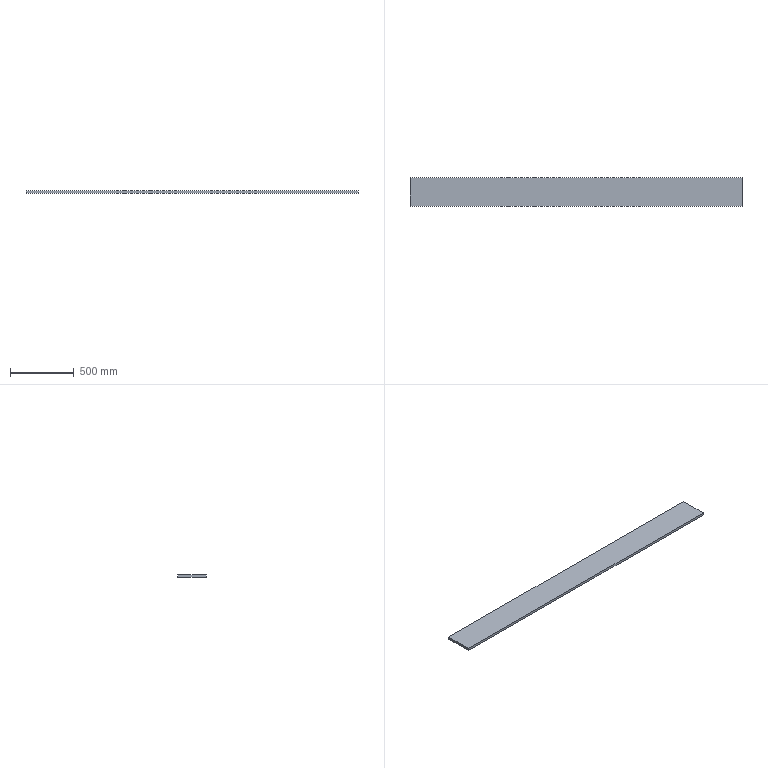Part | NX | features BREP 1, DATUM_CSYS 1, SKETCH 1 | 1 solid | 6 faces | box 2607 x 220 x 20 mm | volume 11470800 mm3 | plane 6
STEP:
#1=CARTESIAN_POINT('',(-1303.5,110.,-10.));
#2=VERTEX_POINT('',#1);
#3=CARTESIAN_POINT('',(-1303.5,-110.,-10.));
#4=VERTEX_POINT('',#3);
#5=CARTESIAN_POINT('',(-1303.5,110.,-10.));
#6=DIRECTION('',(0.,-1.,0.));
#7=VECTOR('',#6,1000.);
#8=LINE('',#5,#7);
#9=EDGE_CURVE('',#2,#4,#8,.T.);
#10=ORIENTED_EDGE('',*,*,#9,.T.);
#11=CARTESIAN_POINT('',(-1303.5,-110.,10.));
#12=VERTEX_POINT('',#11);
#13=CARTESIAN_POINT('',(-1303.5,-110.,10.));
#14=DIRECTION('',(0.,0.,-1.));
#15=VECTOR('',#14,1000.);
#16=LINE('',#13,#15);
#17=EDGE_CURVE('',#12,#4,#16,.T.);
#18=ORIENTED_EDGE('',*,*,#17,.F.);
#19=CARTESIAN_POINT('',(-1303.5,110.,10.));
#20=VERTEX_POINT('',#19);
#21=CARTESIAN_POINT('',(-1303.5,110.,10.));
#22=DIRECTION('',(0.,-1.,0.));
#23=VECTOR('',#22,1000.);
#24=LINE('',#21,#23);
#25=EDGE_CURVE('',#20,#12,#24,.T.);
#26=ORIENTED_EDGE('',*,*,#25,.F.);
#27=CARTESIAN_POINT('',(-1303.5,110.,10.));
#28=DIRECTION('',(0.,0.,-1.));
#29=VECTOR('',#28,1000.);
#30=LINE('',#27,#29);
#31=EDGE_CURVE('',#20,#2,#30,.T.);
#32=ORIENTED_EDGE('',*,*,#31,.T.);
#33=EDGE_LOOP('',(#10,#18,#26,#32));
#34=FACE_BOUND('',#33,.T.);
#35=CARTESIAN_POINT('',(-1303.5,110.,10.));
#36=DIRECTION('',(1.,0.,0.));
#37=DIRECTION('',(0.,0.,1.));
#38=AXIS2_PLACEMENT_3D('',#35,#36,#37);
#39=PLANE('',#38);
#40=ADVANCED_FACE('',(#34),#39,.F.);
#41=CARTESIAN_POINT('',(1303.5,-110.,-10.));
#42=VERTEX_POINT('',#41);
#43=CARTESIAN_POINT('',(-1303.5,-110.,-10.));
#44=DIRECTION('',(1.,0.,0.));
#45=VECTOR('',#44,1000.);
#46=LINE('',#43,#45);
#47=EDGE_CURVE('',#4,#42,#46,.T.);
#48=ORIENTED_EDGE('',*,*,#47,.T.);
#49=CARTESIAN_POINT('',(1303.5,-110.,10.));
#50=VERTEX_POINT('',#49);
#51=CARTESIAN_POINT('',(1303.5,-110.,10.));
#52=DIRECTION('',(0.,0.,-1.));
#53=VECTOR('',#52,1000.);
#54=LINE('',#51,#53);
#55=EDGE_CURVE('',#50,#42,#54,.T.);
#56=ORIENTED_EDGE('',*,*,#55,.F.);
#57=CARTESIAN_POINT('',(-1303.5,-110.,10.));
#58=DIRECTION('',(1.,0.,0.));
#59=VECTOR('',#58,1000.);
#60=LINE('',#57,#59);
#61=EDGE_CURVE('',#12,#50,#60,.T.);
#62=ORIENTED_EDGE('',*,*,#61,.F.);
#63=ORIENTED_EDGE('',*,*,#17,.T.);
#64=EDGE_LOOP('',(#48,#56,#62,#63));
#65=FACE_BOUND('',#64,.T.);
#66=CARTESIAN_POINT('',(-1303.5,-110.,10.));
#67=DIRECTION('',(0.,1.,0.));
#68=DIRECTION('',(0.,0.,-1.));
#69=AXIS2_PLACEMENT_3D('',#66,#67,#68);
#70=PLANE('',#69);
#71=ADVANCED_FACE('',(#65),#70,.F.);
#72=CARTESIAN_POINT('',(1303.5,110.,-10.));
#73=VERTEX_POINT('',#72);
#74=CARTESIAN_POINT('',(1303.5,110.,-10.));
#75=DIRECTION('',(0.,1.,0.));
#76=VECTOR('',#75,1000.);
#77=LINE('',#74,#76);
#78=EDGE_CURVE('',#42,#73,#77,.T.);
#79=ORIENTED_EDGE('',*,*,#78,.T.);
#80=CARTESIAN_POINT('',(1303.5,110.,10.));
#81=VERTEX_POINT('',#80);
#82=CARTESIAN_POINT('',(1303.5,110.,10.));
#83=DIRECTION('',(0.,0.,-1.));
#84=VECTOR('',#83,1000.);
#85=LINE('',#82,#84);
#86=EDGE_CURVE('',#81,#73,#85,.T.);
#87=ORIENTED_EDGE('',*,*,#86,.F.);
#88=CARTESIAN_POINT('',(1303.5,110.,10.));
#89=DIRECTION('',(0.,1.,0.));
#90=VECTOR('',#89,1000.);
#91=LINE('',#88,#90);
#92=EDGE_CURVE('',#50,#81,#91,.T.);
#93=ORIENTED_EDGE('',*,*,#92,.F.);
#94=ORIENTED_EDGE('',*,*,#55,.T.);
#95=EDGE_LOOP('',(#79,#87,#93,#94));
#96=FACE_BOUND('',#95,.T.);
#97=CARTESIAN_POINT('',(1303.5,110.,10.));
#98=DIRECTION('',(-1.,0.,0.));
#99=DIRECTION('',(0.,0.,-1.));
#100=AXIS2_PLACEMENT_3D('',#97,#98,#99);
#101=PLANE('',#100);
#102=ADVANCED_FACE('',(#96),#101,.F.);
#103=CARTESIAN_POINT('',(-1303.5,110.,-10.));
#104=DIRECTION('',(-1.,0.,0.));
#105=VECTOR('',#104,1000.);
#106=LINE('',#103,#105);
#107=EDGE_CURVE('',#73,#2,#106,.T.);
#108=ORIENTED_EDGE('',*,*,#107,.T.);
#109=ORIENTED_EDGE('',*,*,#31,.F.);
#110=CARTESIAN_POINT('',(-1303.5,110.,10.));
#111=DIRECTION('',(-1.,0.,0.));
#112=VECTOR('',#111,1000.);
#113=LINE('',#110,#112);
#114=EDGE_CURVE('',#81,#20,#113,.T.);
#115=ORIENTED_EDGE('',*,*,#114,.F.);
#116=ORIENTED_EDGE('',*,*,#86,.T.);
#117=EDGE_LOOP('',(#108,#109,#115,#116));
#118=FACE_BOUND('',#117,.T.);
#119=CARTESIAN_POINT('',(-1303.5,110.,10.));
#120=DIRECTION('',(0.,-1.,0.));
#121=DIRECTION('',(0.,0.,1.));
#122=AXIS2_PLACEMENT_3D('',#119,#120,#121);
#123=PLANE('',#122);
#124=ADVANCED_FACE('',(#118),#123,.F.);
#125=ORIENTED_EDGE('',*,*,#25,.T.);
#126=ORIENTED_EDGE('',*,*,#61,.T.);
#127=ORIENTED_EDGE('',*,*,#92,.T.);
#128=ORIENTED_EDGE('',*,*,#114,.T.);
#129=EDGE_LOOP('',(#125,#126,#127,#128));
#130=FACE_BOUND('',#129,.T.);
#131=CARTESIAN_POINT('',(-1303.5,-110.,10.));
#132=DIRECTION('',(0.,0.,1.));
#133=DIRECTION('',(-1.,0.,0.));
#134=AXIS2_PLACEMENT_3D('',#131,#132,#133);
#135=PLANE('',#134);
#136=ADVANCED_FACE('',(#130),#135,.T.);
#137=ORIENTED_EDGE('',*,*,#9,.F.);
#138=ORIENTED_EDGE('',*,*,#107,.F.);
#139=ORIENTED_EDGE('',*,*,#78,.F.);
#140=ORIENTED_EDGE('',*,*,#47,.F.);
#141=EDGE_LOOP('',(#137,#138,#139,#140));
#142=FACE_BOUND('',#141,.T.);
#143=CARTESIAN_POINT('',(-1303.5,-110.,-10.));
#144=DIRECTION('',(0.,0.,1.));
#145=DIRECTION('',(-1.,0.,0.));
#146=AXIS2_PLACEMENT_3D('',#143,#144,#145);
#147=PLANE('',#146);
#148=ADVANCED_FACE('',(#142),#147,.F.);
#149=CLOSED_SHELL('',(#40,#71,#102,#124,#136,#148));
#150=MANIFOLD_SOLID_BREP('',#149);
#151=(LENGTH_UNIT()NAMED_UNIT(*)SI_UNIT(.MILLI.,.METRE.));
#152=UNCERTAINTY_MEASURE_WITH_UNIT(LENGTH_MEASURE(0.00001),#151,'','');
#153=(NAMED_UNIT(*)PLANE_ANGLE_UNIT()SI_UNIT($,.RADIAN.));
#154=(NAMED_UNIT(*)SI_UNIT($,.STERADIAN.)SOLID_ANGLE_UNIT());
#155=(GEOMETRIC_REPRESENTATION_CONTEXT(3)GLOBAL_UNCERTAINTY_ASSIGNED_CONTEXT((#152))GLOBAL_UNIT_ASSIGNED_CONTEXT((#151,#153,#154))REPRESENTATION_CONTEXT('',''));
#156=ADVANCED_BREP_SHAPE_REPRESENTATION('',(#150),#155);